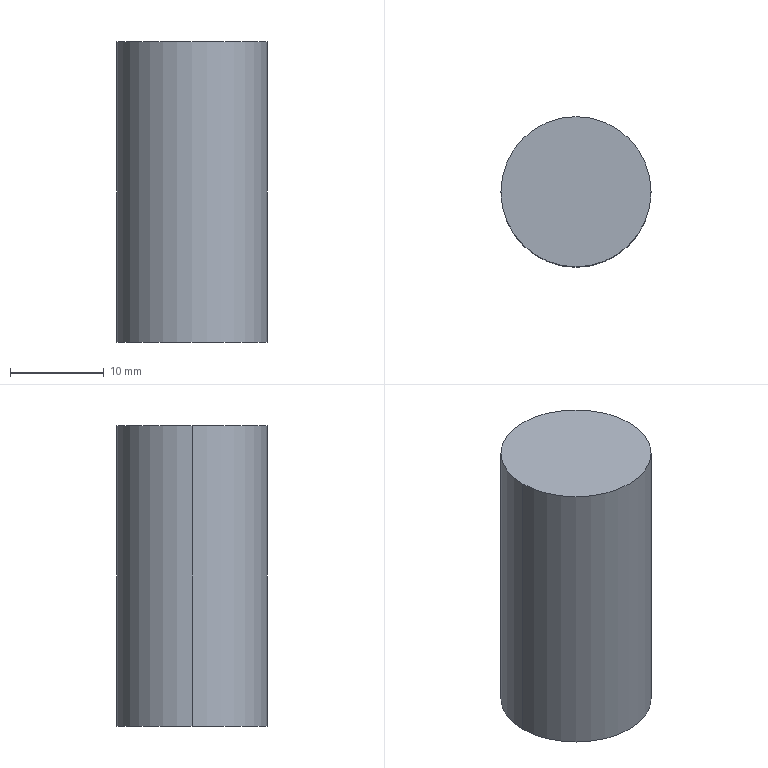Part | SolidWorks | features Extrusion 1 | 1 solid | 4 faces | box 16 x 16 x 32 mm | volume 6434 mm3 | cylinder 2 | plane 2 | commonest cylinder face diameters 16 x2
STEP:
#1=CARTESIAN_POINT('',(8.,0.,-16.));
#2=VERTEX_POINT('',#1);
#3=CARTESIAN_POINT('',(-8.,0.,-16.));
#4=VERTEX_POINT('',#3);
#5=CARTESIAN_POINT('',(0.,0.,-16.));
#6=DIRECTION('',(0.,0.,1.));
#7=DIRECTION('',(1.,0.,0.));
#8=AXIS2_PLACEMENT_3D('',#5,#6,#7);
#9=CIRCLE('',#8,8.);
#10=EDGE_CURVE('',#2,#4,#9,.T.);
#11=ORIENTED_EDGE('',*,*,#10,.T.);
#12=CARTESIAN_POINT('',(-8.,0.,16.));
#13=VERTEX_POINT('',#12);
#14=CARTESIAN_POINT('',(-8.,0.,-16.));
#15=DIRECTION('',(0.,0.,1.));
#16=VECTOR('',#15,1000.);
#17=LINE('',#14,#16);
#18=EDGE_CURVE('',#4,#13,#17,.T.);
#19=ORIENTED_EDGE('',*,*,#18,.T.);
#20=CARTESIAN_POINT('',(8.,0.,16.));
#21=VERTEX_POINT('',#20);
#22=CARTESIAN_POINT('',(0.,0.,16.));
#23=DIRECTION('',(0.,0.,1.));
#24=DIRECTION('',(1.,0.,0.));
#25=AXIS2_PLACEMENT_3D('',#22,#23,#24);
#26=CIRCLE('',#25,8.);
#27=EDGE_CURVE('',#21,#13,#26,.T.);
#28=ORIENTED_EDGE('',*,*,#27,.F.);
#29=CARTESIAN_POINT('',(8.,0.,-16.));
#30=DIRECTION('',(0.,0.,1.));
#31=VECTOR('',#30,1000.);
#32=LINE('',#29,#31);
#33=EDGE_CURVE('',#2,#21,#32,.T.);
#34=ORIENTED_EDGE('',*,*,#33,.F.);
#35=EDGE_LOOP('',(#11,#19,#28,#34));
#36=FACE_OUTER_BOUND('',#35,.T.);
#37=CARTESIAN_POINT('',(0.,0.,-16.));
#38=DIRECTION('',(0.,0.,1.));
#39=DIRECTION('',(1.,0.,0.));
#40=AXIS2_PLACEMENT_3D('',#37,#38,#39);
#41=CYLINDRICAL_SURFACE('',#40,8.);
#42=ADVANCED_FACE('',(#36),#41,.T.);
#43=ORIENTED_EDGE('',*,*,#18,.F.);
#44=CARTESIAN_POINT('',(0.,0.,-16.));
#45=DIRECTION('',(0.,0.,1.));
#46=DIRECTION('',(1.,0.,0.));
#47=AXIS2_PLACEMENT_3D('',#44,#45,#46);
#48=CIRCLE('',#47,8.);
#49=EDGE_CURVE('',#4,#2,#48,.T.);
#50=ORIENTED_EDGE('',*,*,#49,.T.);
#51=ORIENTED_EDGE('',*,*,#33,.T.);
#52=CARTESIAN_POINT('',(0.,0.,16.));
#53=DIRECTION('',(0.,0.,1.));
#54=DIRECTION('',(1.,0.,0.));
#55=AXIS2_PLACEMENT_3D('',#52,#53,#54);
#56=CIRCLE('',#55,8.);
#57=EDGE_CURVE('',#13,#21,#56,.T.);
#58=ORIENTED_EDGE('',*,*,#57,.F.);
#59=EDGE_LOOP('',(#43,#50,#51,#58));
#60=FACE_OUTER_BOUND('',#59,.T.);
#61=CARTESIAN_POINT('',(0.,0.,-16.));
#62=DIRECTION('',(0.,0.,1.));
#63=DIRECTION('',(1.,0.,0.));
#64=AXIS2_PLACEMENT_3D('',#61,#62,#63);
#65=CYLINDRICAL_SURFACE('',#64,8.);
#66=ADVANCED_FACE('',(#60),#65,.T.);
#67=ORIENTED_EDGE('',*,*,#10,.F.);
#68=ORIENTED_EDGE('',*,*,#49,.F.);
#69=EDGE_LOOP('',(#67,#68));
#70=FACE_OUTER_BOUND('',#69,.T.);
#71=CARTESIAN_POINT('',(0.,0.,-16.));
#72=DIRECTION('',(0.,0.,1.));
#73=DIRECTION('',(1.,0.,0.));
#74=AXIS2_PLACEMENT_3D('',#71,#72,#73);
#75=PLANE('',#74);
#76=ADVANCED_FACE('',(#70),#75,.F.);
#77=ORIENTED_EDGE('',*,*,#27,.T.);
#78=ORIENTED_EDGE('',*,*,#57,.T.);
#79=EDGE_LOOP('',(#77,#78));
#80=FACE_OUTER_BOUND('',#79,.T.);
#81=CARTESIAN_POINT('',(0.,0.,16.));
#82=DIRECTION('',(0.,0.,1.));
#83=DIRECTION('',(1.,0.,0.));
#84=AXIS2_PLACEMENT_3D('',#81,#82,#83);
#85=PLANE('',#84);
#86=ADVANCED_FACE('',(#80),#85,.T.);
#87=CLOSED_SHELL('',(#42,#66,#76,#86));
#88=MANIFOLD_SOLID_BREP('',#87);
#89=CARTESIAN_POINT('',(0.,0.,0.));
#90=DIRECTION('',(0.,0.,1.));
#91=DIRECTION('',(1.,0.,0.));
#92=AXIS2_PLACEMENT_3D('',#89,#90,#91);
#93=(LENGTH_UNIT()NAMED_UNIT(*)SI_UNIT(.MILLI.,.METRE.));
#94=UNCERTAINTY_MEASURE_WITH_UNIT(LENGTH_MEASURE(0.00001),#93,'','');
#95=(NAMED_UNIT(*)PLANE_ANGLE_UNIT()SI_UNIT($,.RADIAN.));
#96=(NAMED_UNIT(*)SI_UNIT($,.STERADIAN.)SOLID_ANGLE_UNIT());
#97=(GEOMETRIC_REPRESENTATION_CONTEXT(3)GLOBAL_UNCERTAINTY_ASSIGNED_CONTEXT((#94))GLOBAL_UNIT_ASSIGNED_CONTEXT((#93,#95,#96))REPRESENTATION_CONTEXT('',''));
#98=ADVANCED_BREP_SHAPE_REPRESENTATION('',(#88,#92),#97);